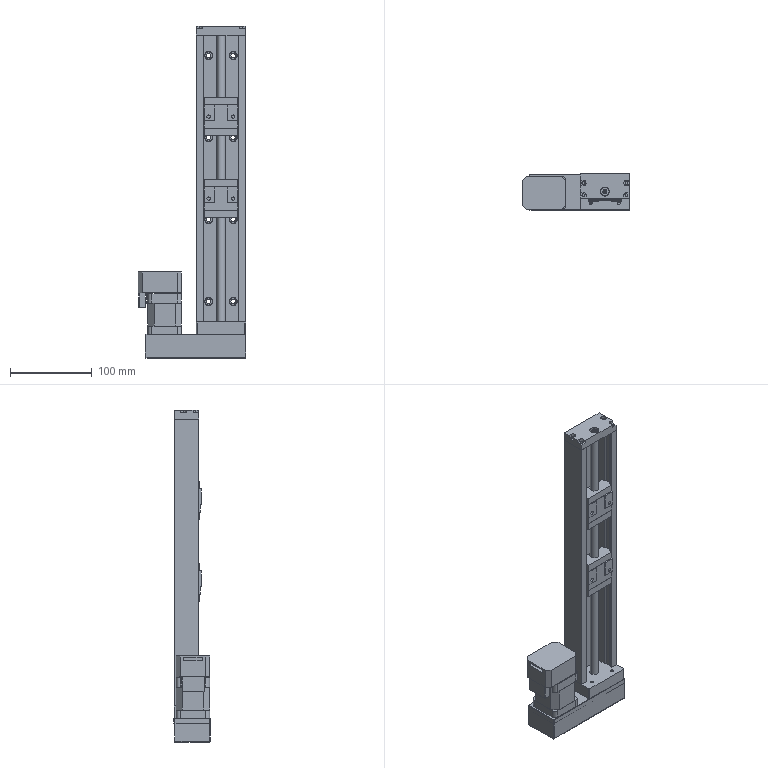Part | SolidWorks | 13 solids | 419 faces | box 131.635 x 44 x 404.935 mm | volume 615573 mm3 | plane 199 | cylinder 187 | cone 28 | spline 5 | commonest cylinder face diameters 3.5 x16 5.5 x16 9 x16 4 x14 10 x12 30 x10